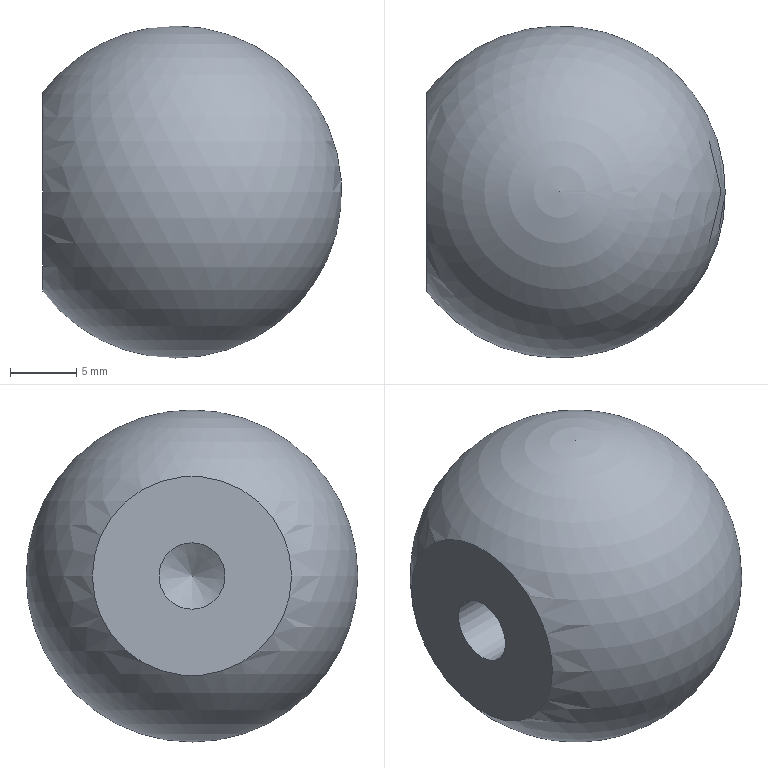Part | NX | features BREP 1 | 1 solid | 4 faces | box 22.5 x 25 x 25 mm | volume 7648 mm3 | sphere 1 | plane 1 | cone 1 | cylinder 1 | commonest cylinder face diameters 5 x1
STEP:
#1=CARTESIAN_POINT('',(-10.,7.5,0.));
#2=VERTEX_POINT('',#1);
#3=CARTESIAN_POINT('',(-10.,0.,0.));
#4=DIRECTION('',(-1.,0.,0.));
#5=DIRECTION('',(0.,1.,0.));
#6=AXIS2_PLACEMENT_3D('',#3,#4,#5);
#7=CIRCLE('',#6,7.5);
#8=EDGE_CURVE('',#2,#2,#7,.T.);
#9=ORIENTED_EDGE('',*,*,#8,.F.);
#10=EDGE_LOOP('',(#9));
#11=FACE_BOUND('',#10,.T.);
#12=CARTESIAN_POINT('',(0.,0.,0.));
#13=DIRECTION('',(0.,0.,-1.));
#14=DIRECTION('',(-1.,0.,0.));
#15=AXIS2_PLACEMENT_3D('',#12,#13,#14);
#16=SPHERICAL_SURFACE('',#15,12.5);
#17=ADVANCED_FACE('',(#11),#16,.T.);
#18=CARTESIAN_POINT('',(-10.,0.,2.5));
#19=VERTEX_POINT('',#18);
#20=CARTESIAN_POINT('',(-10.,0.,0.));
#21=DIRECTION('',(-1.,0.,0.));
#22=DIRECTION('',(0.,0.,1.));
#23=AXIS2_PLACEMENT_3D('',#20,#21,#22);
#24=CIRCLE('',#23,2.5);
#25=EDGE_CURVE('',#19,#19,#24,.T.);
#26=ORIENTED_EDGE('',*,*,#25,.F.);
#27=EDGE_LOOP('',(#26));
#28=FACE_BOUND('',#27,.T.);
#29=ORIENTED_EDGE('',*,*,#8,.T.);
#30=EDGE_LOOP('',(#29));
#31=FACE_BOUND('',#30,.T.);
#32=CARTESIAN_POINT('',(-10.,13.905,-12.5));
#33=DIRECTION('',(1.,0.,0.));
#34=DIRECTION('',(0.,-1.,0.));
#35=AXIS2_PLACEMENT_3D('',#32,#33,#34);
#36=PLANE('',#35);
#37=ADVANCED_FACE('',(#28,#31),#36,.F.);
#38=CARTESIAN_POINT('',(6.502,0.,0.));
#39=VERTEX_POINT('',#38);
#40=VERTEX_LOOP('',#39);
#41=FACE_BOUND('',#40,.T.);
#42=CARTESIAN_POINT('',(5.,0.,2.5));
#43=VERTEX_POINT('',#42);
#44=CARTESIAN_POINT('',(5.,0.,0.));
#45=DIRECTION('',(-1.,0.,0.));
#46=DIRECTION('',(0.,0.,1.));
#47=AXIS2_PLACEMENT_3D('',#44,#45,#46);
#48=CIRCLE('',#47,2.5);
#49=EDGE_CURVE('',#43,#43,#48,.T.);
#50=ORIENTED_EDGE('',*,*,#49,.T.);
#51=EDGE_LOOP('',(#50));
#52=FACE_BOUND('',#51,.T.);
#53=CARTESIAN_POINT('',(5.,0.,0.));
#54=DIRECTION('',(-1.,0.,0.));
#55=DIRECTION('',(0.,0.,-1.));
#56=AXIS2_PLACEMENT_3D('',#53,#54,#55);
#57=CONICAL_SURFACE('',#56,2.5,1.03);
#58=ADVANCED_FACE('',(#41,#52),#57,.F.);
#59=ORIENTED_EDGE('',*,*,#49,.F.);
#60=EDGE_LOOP('',(#59));
#61=FACE_BOUND('',#60,.T.);
#62=ORIENTED_EDGE('',*,*,#25,.T.);
#63=EDGE_LOOP('',(#62));
#64=FACE_BOUND('',#63,.T.);
#65=CARTESIAN_POINT('',(-10.,0.,0.));
#66=DIRECTION('',(-1.,0.,0.));
#67=DIRECTION('',(0.,0.,-1.));
#68=AXIS2_PLACEMENT_3D('',#65,#66,#67);
#69=CYLINDRICAL_SURFACE('',#68,2.5);
#70=ADVANCED_FACE('',(#61,#64),#69,.F.);
#71=CLOSED_SHELL('',(#17,#37,#58,#70));
#72=MANIFOLD_SOLID_BREP('',#71);
#73=(LENGTH_UNIT()NAMED_UNIT(*)SI_UNIT(.MILLI.,.METRE.));
#74=UNCERTAINTY_MEASURE_WITH_UNIT(LENGTH_MEASURE(0.00001),#73,'','');
#75=(NAMED_UNIT(*)PLANE_ANGLE_UNIT()SI_UNIT($,.RADIAN.));
#76=(NAMED_UNIT(*)SI_UNIT($,.STERADIAN.)SOLID_ANGLE_UNIT());
#77=(GEOMETRIC_REPRESENTATION_CONTEXT(3)GLOBAL_UNCERTAINTY_ASSIGNED_CONTEXT((#74))GLOBAL_UNIT_ASSIGNED_CONTEXT((#73,#75,#76))REPRESENTATION_CONTEXT('',''));
#78=ADVANCED_BREP_SHAPE_REPRESENTATION('',(#72),#77);